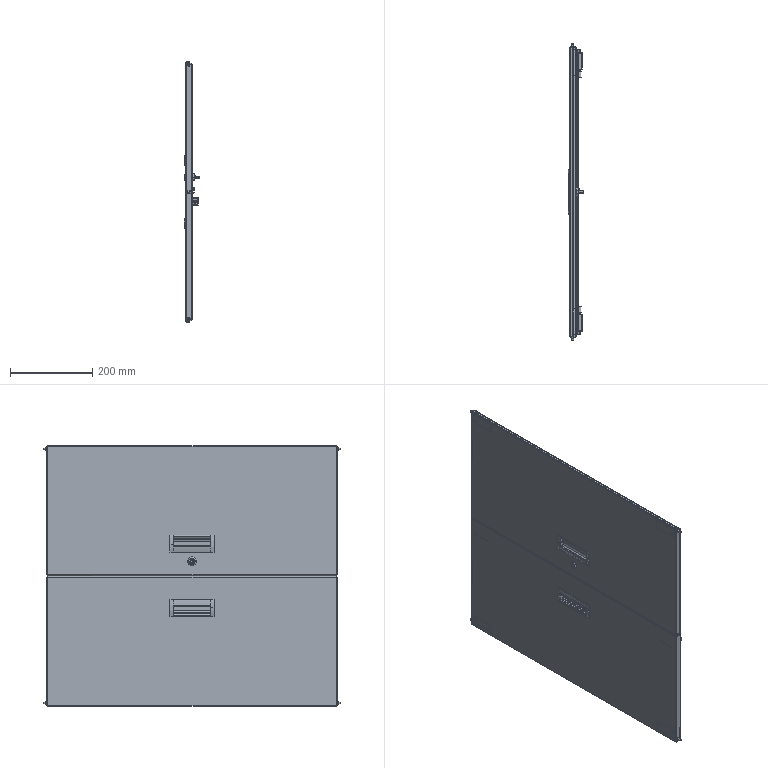Part | SolidWorks | 25 solids | 704 faces | box 37.5 x 724 x 636 mm | volume 879257 mm3 | plane 394 | cylinder 280 | cone 14 | torus 8 | spline 8 | commonest cylinder face diameters 1 x36 7 x23 0.6 x21 2.5 x16 3.2 x16 5.5 x16